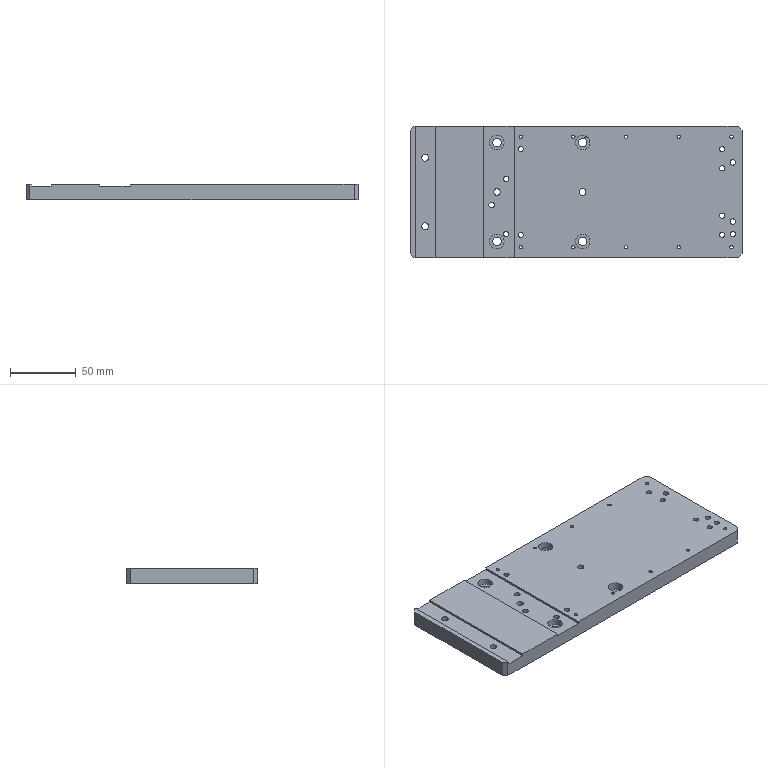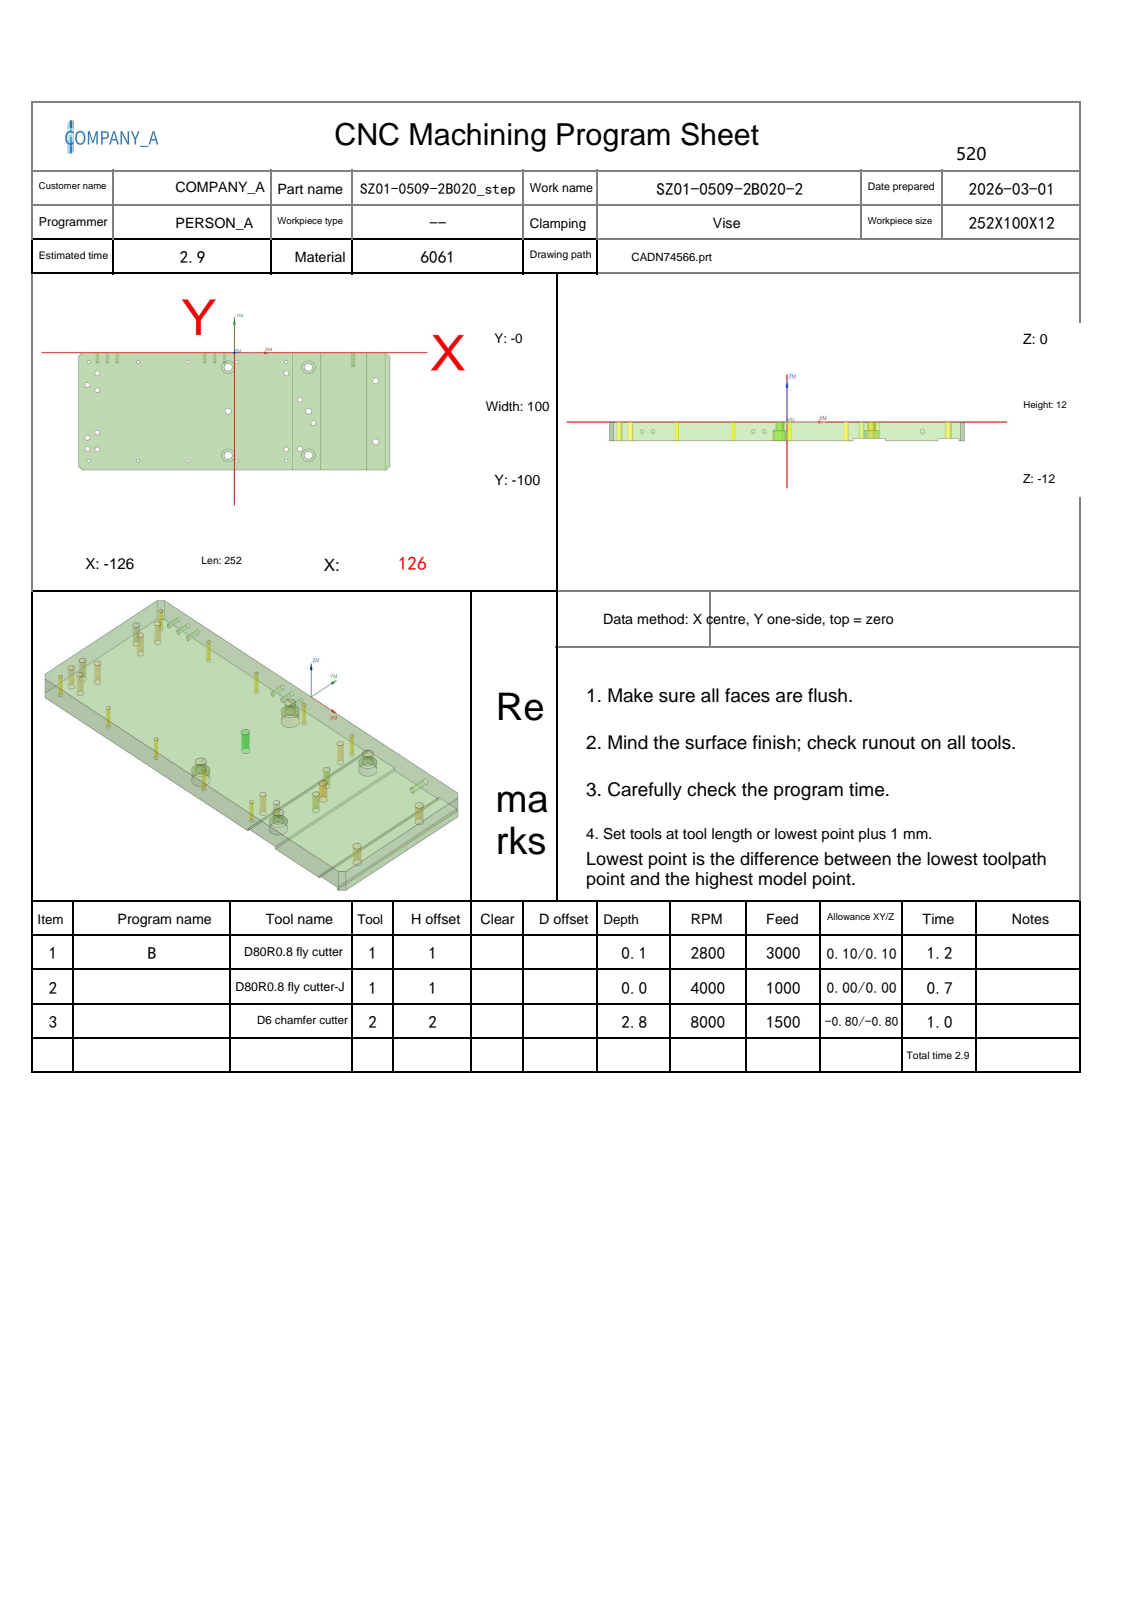NC program | NX | posted by the shop | part box 252 x 100 x 12 mm
Whole program:
%
O0001
(Machine time: 3.55 MIN)
(===Total Tool:2===)
(T1=D80R0.8 fly cutter D=80.  R=0.8  D-  H01 Z=0.    )
(T2=D6 chamfer cutter   D=6.   R=0.   D-  H02 Z=-2.8  )
G80 G90 G17 G49 G40
G91 G28 Z0
M01
N1 T01 M06
(D80R0.8 fly cutter  D=80. R=0.8 H=01 ce=0.10 di=0.10)
G00 G90 G54 X-178.097 Y-23.903 M03 S2800
G43 H01 Z50.
M08
Z4.02
G01 Z2.02 F3000.
X-166.097
X158.897
G02 X166.097 Y-31.103 I0.0 J-7.2
G01 Y-60.737
G02 X158.097 Y-68.737 I-8. J0.0
G01 X-166.097
X-178.097
Z4.02
G00 Y-23.903
Z3.54
G01 Z1.54
X-166.097
X158.897
G02 X166.097 Y-31.103 I0.0 J-7.2
G01 Y-60.737
G02 X158.097 Y-68.737 I-8. J0.0
G01 X-166.097
X-178.097
Z3.54
G00 Y-23.903
Z3.06
G01 Z1.06
X-166.097
X158.897
G02 X166.097 Y-31.103 I0.0 J-7.2
G01 Y-60.737
G02 X158.097 Y-68.737 I-8. J0.0
G01 X-166.097
X-178.097
Z3.06
G00 Y-23.903
Z2.58
G01 Z.58
X-166.097
X158.897
G02 X166.097 Y-31.103 I0.0 J-7.2
G01 Y-60.737
G02 X158.097 Y-68.737 I-8. J0.0
G01 X-166.097
X-178.097
Z2.58
G00 Y-23.903
Z2.1
G01 Z.1
X-166.097
X158.897
G02 X166.097 Y-31.103 I0.0 J-7.2
G01 Y-60.737
G02 X158.097 Y-68.737 I-8. J0.0
G01 X-166.097
X-178.097
Z2.1
G00 Z50.
G91 G28 Z0.0
M05
M09
G91 G28 Z0.0
M01
N2 T01 M06
(D80R0.8 fly cutter-J  D=80. R=0.8 H=01 ce=0.00 di=0.00)
G00 G90 G54 X-177.999 Y-24.001 M03 S4000
G43 H01 Z50.
M08
Z2.
G01 Z0.0 F1000.
X-165.999
X158.799
G02 X165.999 Y-31.201 I0.0 J-7.2
G01 Y-60.639
G02 X157.999 Y-68.639 I-8. J0.0
G01 X-165.999
X-177.999
Z2.
G00 Z50.
G91 G28 Z0.0
M05
M09
G91 G28 Z0.0
M01
N3 T02 M06
(D6 chamfer cutter  D=6. R=0. H=02 ce=0.00 di=0.00)
G00 G90 G54 X42. Y-8. M03 S8000
G43 H02 Z50.
M08
G98 G81 X42. Y-8. Z-1.75 R3. F1000.
X2.
X-38.
X-78.
X-118.
Y-92.
X-78.
X-38.
X2.
X42.
G80
G00 Z50.
G00 G90 X-119. Y-82. M03 S8000
Z50.
G98 G81 X-119. Y-82. Z-2.3 R3. F1000.
X-111. Y-82.5
Y-68.
Y-32.
Y-17.5
X42.
Y-82.5
X53. Y-82.
G80
G00 Z50.
G00 G90 X-5. Y-50. M03 S8000
Z50.
G98 G81 X-5. Y-50. Z-2.8 R3. F1000.
X60.
G80
G00 Z50.
G00 G90 X-119. Y-72.5 M03 S8000
Z50.
G98 G81 X-119. Y-72.5 Z-2.7 R3. F1000.
Y-27.5
X53. Y-40.
X64. Y-60.
G80
G00 Z50.
G00 G90 X114.773 Y-24.91 M03 S8000
Z50.
Z-.9
G01 Z-1.4 F600.
X114.95 Y-25.5
G03 X116.45 Y-24. I0.0 J1.5
X114.5 Y-22.05 I-1.95 J0.0
X112.55 Y-24. I0.0 J-1.95
X114.5 Y-25.95 I1.95 J0.0
X116.45 Y-24. I0.0 J1.95
X114.95 Y-22.5 I-1.5 J0.0
G01 X114.773 Y-23.09
Z-.9
G00 Z50.
Y-76.91
Z-.9
G01 Z-1.4
X114.95 Y-77.5
G03 X116.45 Y-76. I0.0 J1.5
X114.5 Y-74.05 I-1.95 J0.0
X112.55 Y-76. I0.0 J-1.95
X114.5 Y-77.95 I1.95 J0.0
X116.45 Y-76. I0.0 J1.95
X114.95 Y-74.5 I-1.5 J0.0
G01 X114.773 Y-75.09
Z-.9
G00 Z50.
G00 G90 X-4.493 Y-13.587 M03 S8000
Z50.
Z-.9
G01 Z-1.4 F1200.
X-4.3 Y-14.
G03 X-2.8 Y-12.5 I0.0 J1.5
X-5. Y-10.3 I-2.2 J0.0
X-7.2 Y-12.5 I0.0 J-2.2
X-5. Y-14.7 I2.2 J0.0
X-2.8 Y-12.5 I0.0 J2.2
X-4.3 Y-11. I-1.5 J0.0
G01 X-4.493 Y-11.413
Z-.9
G00 Z50.
X60.507 Y-13.587
Z-.9
G01 Z-1.4
X60.7 Y-14.
G03 X62.2 Y-12.5 I0.0 J1.5
X60. Y-10.3 I-2.2 J0.0
X57.8 Y-12.5 I0.0 J-2.2
X60. Y-14.7 I2.2 J0.0
X62.2 Y-12.5 I0.0 J2.2
X60.7 Y-11. I-1.5 J0.0
G01 X60.507 Y-11.413
Z-.9
G00 Z50.
Y-88.587
Z-.9
G01 Z-1.4
X60.7 Y-89.
G03 X62.2 Y-87.5 I0.0 J1.5
X60. Y-85.3 I-2.2 J0.0
X57.8 Y-87.5 I0.0 J-2.2
X60. Y-89.7 I2.2 J0.0
X62.2 Y-87.5 I0.0 J2.2
X60.7 Y-86. I-1.5 J0.0
G01 X60.507 Y-86.413
Z-.9
G00 Z50.
X-4.493 Y-88.587
Z-.9
G01 Z-1.4
X-4.3 Y-89.
G03 X-2.8 Y-87.5 I0.0 J1.5
X-5. Y-85.3 I-2.2 J0.0
X-7.2 Y-87.5 I0.0 J-2.2
X-5. Y-89.7 I2.2 J0.0
X-2.8 Y-87.5 I0.0 J2.2
X-4.3 Y-86. I-1.5 J0.0
G01 X-4.493 Y-86.413
Z-.9
G00 Z50.
G00 G90 X-114.046 Y-100.7 M03 S7000
Z50.
Z2.5
G01 X-122.876 Z-.714 F1500.
X-122.953 Z-.742
X-123.16 Y-100.662 Z-.819
X-123.355 Y-100.581 Z-.895
X-123.528 Y-100.462 Z-.972
X-123.583 Y-100.407 Z-1.
X-126.407 Y-97.583
G02 X-126.7 Y-96.876 I.707 J.707
G01 Y-3.124
G02 X-126.407 Y-2.417 I1. J0.0
G01 X-123.583 Y.407
G02 X-122.876 Y.7 I.707 J-.707
G01 X122.876
G02 X123.583 Y.407 I0.0 J-1.
G01 X126.407 Y-2.417
G02 X126.7 Y-3.124 I-.707 J-.707
G01 Y-96.876
G02 X126.407 Y-97.583 I-1. J0.0
G01 X123.583 Y-100.407
G02 X122.876 Y-100.7 I-.707 J.707
G01 X-122.876
G02 X-123.583 Y-100.407 I0.0 J1.
G01 X-123.936 Y-100.054
Z1.5
G00 Z50.
M05
M09
G91 G28 Z0.0
G91 G28 Y0.0
M30
%